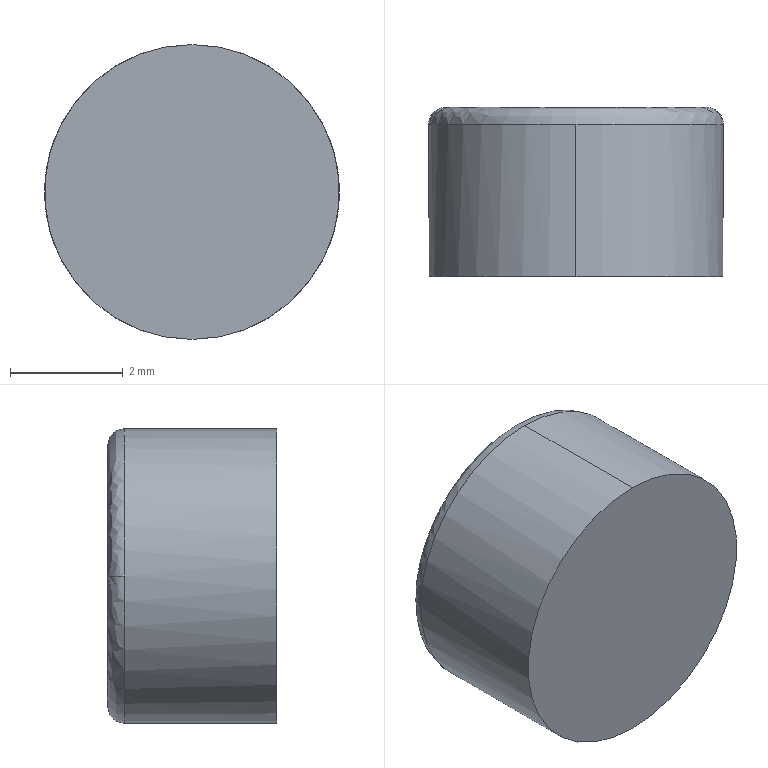Part | SolidWorks | features BaseBody 1 | 1 solid | 19 faces | box 5.232 x 3 x 5.232 mm | volume 54.683 mm3 | plane 15 | spline 2 | cylinder 2 | commonest cylinder face diameters 5.232 x2
STEP:
#1=CARTESIAN_POINT('',(15.184,100.1,10.6));
#2=VERTEX_POINT('',#1);
#3=CARTESIAN_POINT('',(19.816,100.1,10.6));
#4=VERTEX_POINT('',#3);
#5=CARTESIAN_POINT('',(15.184,100.1,10.6));
#6=CARTESIAN_POINT('',(15.184,100.1,5.968));
#7=CARTESIAN_POINT('',(19.816,100.1,5.968));
#8=CARTESIAN_POINT('',(19.816,100.1,10.6));
#9=(BOUNDED_CURVE()B_SPLINE_CURVE(3,(#5,#6,#7,#8),.UNSPECIFIED.,.F.,.T.)B_SPLINE_CURVE_WITH_KNOTS((4,4),(0.,1.),.UNSPECIFIED.)CURVE()GEOMETRIC_REPRESENTATION_ITEM()RATIONAL_B_SPLINE_CURVE((1.,0.3333,0.3333,1.))REPRESENTATION_ITEM(''));
#10=EDGE_CURVE('',#2,#4,#9,.T.);
#11=ORIENTED_EDGE('',*,*,#10,.T.);
#12=CARTESIAN_POINT('',(20.116,99.8,10.6));
#13=VERTEX_POINT('',#12);
#14=CARTESIAN_POINT('',(19.816,99.8,10.6));
#15=DIRECTION('',(0.,0.,-1.));
#16=DIRECTION('',(1.,0.,0.));
#17=AXIS2_PLACEMENT_3D('',#14,#15,#16);
#18=CIRCLE('',#17,0.3);
#19=EDGE_CURVE('',#4,#13,#18,.T.);
#20=ORIENTED_EDGE('',*,*,#19,.T.);
#21=CARTESIAN_POINT('',(17.5,99.8,7.984));
#22=VERTEX_POINT('',#21);
#23=CARTESIAN_POINT('',(17.5,99.8,10.6));
#24=DIRECTION('',(0.,-1.,0.));
#25=DIRECTION('',(0.,0.,1.));
#26=AXIS2_PLACEMENT_3D('',#23,#24,#25);
#27=CIRCLE('',#26,2.616);
#28=EDGE_CURVE('',#22,#13,#27,.T.);
#29=ORIENTED_EDGE('',*,*,#28,.F.);
#30=CARTESIAN_POINT('',(14.884,99.8,10.6));
#31=VERTEX_POINT('',#30);
#32=CARTESIAN_POINT('',(17.5,99.8,10.6));
#33=DIRECTION('',(0.,-1.,0.));
#34=DIRECTION('',(0.,0.,1.));
#35=AXIS2_PLACEMENT_3D('',#32,#33,#34);
#36=CIRCLE('',#35,2.616);
#37=EDGE_CURVE('',#31,#22,#36,.T.);
#38=ORIENTED_EDGE('',*,*,#37,.F.);
#39=CARTESIAN_POINT('',(15.184,99.8,10.6));
#40=DIRECTION('',(0.,0.,1.));
#41=DIRECTION('',(-1.,0.,0.));
#42=AXIS2_PLACEMENT_3D('',#39,#40,#41);
#43=CIRCLE('',#42,0.3);
#44=EDGE_CURVE('',#2,#31,#43,.T.);
#45=ORIENTED_EDGE('',*,*,#44,.F.);
#46=EDGE_LOOP('',(#11,#20,#29,#38,#45));
#47=FACE_OUTER_BOUND('',#46,.T.);
#48=CARTESIAN_POINT('',(19.816,100.1,10.6));
#49=CARTESIAN_POINT('',(19.816,100.1,5.968));
#50=CARTESIAN_POINT('',(15.184,100.1,5.968));
#51=CARTESIAN_POINT('',(15.184,100.1,10.6));
#52=CARTESIAN_POINT('',(19.992,100.1,10.6));
#53=CARTESIAN_POINT('',(19.992,100.1,5.617));
#54=CARTESIAN_POINT('',(15.008,100.1,5.617));
#55=CARTESIAN_POINT('',(15.008,100.1,10.6));
#56=CARTESIAN_POINT('',(20.116,99.976,10.6));
#57=CARTESIAN_POINT('',(20.116,99.976,5.368));
#58=CARTESIAN_POINT('',(14.884,99.976,5.368));
#59=CARTESIAN_POINT('',(14.884,99.976,10.6));
#60=CARTESIAN_POINT('',(20.116,99.8,10.6));
#61=CARTESIAN_POINT('',(20.116,99.8,5.368));
#62=CARTESIAN_POINT('',(14.884,99.8,5.368));
#63=CARTESIAN_POINT('',(14.884,99.8,10.6));
#64=(BOUNDED_SURFACE()B_SPLINE_SURFACE(3,3,((#48,#49,#50,#51),(#52,#53,#54,#55),(#56,#57,#58,#59),(#60,#61,#62,#63)),.UNSPECIFIED.,.F.,.F.,.F.)B_SPLINE_SURFACE_WITH_KNOTS((4,4),(4,4),(0.,1.),(0.,1.),.UNSPECIFIED.)GEOMETRIC_REPRESENTATION_ITEM()RATIONAL_B_SPLINE_SURFACE(((1.,0.3333,0.3333,1.),(0.8047,0.2682,0.2682,0.8047),(0.8047,0.2682,0.2682,0.8047),(1.,0.3333,0.3333,1.)))REPRESENTATION_ITEM('')SURFACE());
#65=ADVANCED_FACE('',(#47),#64,.T.);
#66=CARTESIAN_POINT('',(17.5,97.1,13.216));
#67=VERTEX_POINT('',#66);
#68=CARTESIAN_POINT('',(17.5,97.1,7.984));
#69=VERTEX_POINT('',#68);
#70=CARTESIAN_POINT('',(17.5,97.1,10.6));
#71=DIRECTION('',(0.,1.,0.));
#72=DIRECTION('',(0.,0.,1.));
#73=AXIS2_PLACEMENT_3D('',#70,#71,#72);
#74=CIRCLE('',#73,2.616);
#75=EDGE_CURVE('',#67,#69,#74,.T.);
#76=ORIENTED_EDGE('',*,*,#75,.T.);
#77=CARTESIAN_POINT('',(17.5,98.45,7.984));
#78=DIRECTION('',(0.,1.,0.));
#79=VECTOR('',#78,1000.);
#80=LINE('',#77,#79);
#81=EDGE_CURVE('',#69,#22,#80,.T.);
#82=ORIENTED_EDGE('',*,*,#81,.T.);
#83=ORIENTED_EDGE('',*,*,#28,.T.);
#84=CARTESIAN_POINT('',(17.5,99.8,13.216));
#85=VERTEX_POINT('',#84);
#86=CARTESIAN_POINT('',(17.5,99.8,10.6));
#87=DIRECTION('',(0.,-1.,0.));
#88=DIRECTION('',(0.,0.,1.));
#89=AXIS2_PLACEMENT_3D('',#86,#87,#88);
#90=CIRCLE('',#89,2.616);
#91=EDGE_CURVE('',#13,#85,#90,.T.);
#92=ORIENTED_EDGE('',*,*,#91,.T.);
#93=CARTESIAN_POINT('',(17.5,98.45,13.216));
#94=DIRECTION('',(0.,1.,0.));
#95=VECTOR('',#94,1000.);
#96=LINE('',#93,#95);
#97=EDGE_CURVE('',#67,#85,#96,.T.);
#98=ORIENTED_EDGE('',*,*,#97,.F.);
#99=EDGE_LOOP('',(#76,#82,#83,#92,#98));
#100=FACE_OUTER_BOUND('',#99,.T.);
#101=CARTESIAN_POINT('',(17.5,98.45,10.6));
#102=DIRECTION('',(0.,1.,0.));
#103=DIRECTION('',(0.,0.,1.));
#104=AXIS2_PLACEMENT_3D('',#101,#102,#103);
#105=CYLINDRICAL_SURFACE('',#104,2.616);
#106=ADVANCED_FACE('',(#100),#105,.T.);
#107=ORIENTED_EDGE('',*,*,#81,.F.);
#108=CARTESIAN_POINT('',(17.5,97.1,10.6));
#109=DIRECTION('',(0.,1.,0.));
#110=DIRECTION('',(0.,0.,1.));
#111=AXIS2_PLACEMENT_3D('',#108,#109,#110);
#112=CIRCLE('',#111,2.616);
#113=EDGE_CURVE('',#69,#67,#112,.T.);
#114=ORIENTED_EDGE('',*,*,#113,.T.);
#115=ORIENTED_EDGE('',*,*,#97,.T.);
#116=CARTESIAN_POINT('',(17.5,99.8,10.6));
#117=DIRECTION('',(0.,-1.,0.));
#118=DIRECTION('',(0.,0.,1.));
#119=AXIS2_PLACEMENT_3D('',#116,#117,#118);
#120=CIRCLE('',#119,2.616);
#121=EDGE_CURVE('',#85,#31,#120,.T.);
#122=ORIENTED_EDGE('',*,*,#121,.T.);
#123=ORIENTED_EDGE('',*,*,#37,.T.);
#124=EDGE_LOOP('',(#107,#114,#115,#122,#123));
#125=FACE_OUTER_BOUND('',#124,.T.);
#126=CARTESIAN_POINT('',(17.5,98.45,10.6));
#127=DIRECTION('',(0.,1.,0.));
#128=DIRECTION('',(0.,0.,1.));
#129=AXIS2_PLACEMENT_3D('',#126,#127,#128);
#130=CYLINDRICAL_SURFACE('',#129,2.616);
#131=ADVANCED_FACE('',(#125),#130,.T.);
#132=ORIENTED_EDGE('',*,*,#19,.F.);
#133=CARTESIAN_POINT('',(15.184,100.1,10.6));
#134=CARTESIAN_POINT('',(15.184,100.1,10.747));
#135=CARTESIAN_POINT('',(15.204,100.1,10.964));
#136=CARTESIAN_POINT('',(15.264,100.1,11.211));
#137=CARTESIAN_POINT('',(15.302,100.1,11.332));
#138=CARTESIAN_POINT('',(15.321,100.1,11.384));
#139=CARTESIAN_POINT('',(15.333,100.1,11.418));
#140=CARTESIAN_POINT('',(15.339,100.1,11.434));
#141=CARTESIAN_POINT('',(15.464,100.1,11.75));
#142=CARTESIAN_POINT('',(15.637,100.1,12.012));
#143=CARTESIAN_POINT('',(15.975,100.1,12.351));
#144=CARTESIAN_POINT('',(16.158,100.1,12.5));
#145=CARTESIAN_POINT('',(16.395,100.1,12.638));
#146=CARTESIAN_POINT('',(16.519,100.1,12.699));
#147=CARTESIAN_POINT('',(16.574,100.1,12.723));
#148=CARTESIAN_POINT('',(16.61,100.1,12.738));
#149=CARTESIAN_POINT('',(16.63,100.1,12.747));
#150=CARTESIAN_POINT('',(16.921,100.1,12.862));
#151=CARTESIAN_POINT('',(17.206,100.1,12.916));
#152=CARTESIAN_POINT('',(17.647,100.1,12.916));
#153=CARTESIAN_POINT('',(17.864,100.1,12.896));
#154=CARTESIAN_POINT('',(18.11,100.1,12.836));
#155=CARTESIAN_POINT('',(18.232,100.1,12.798));
#156=CARTESIAN_POINT('',(18.284,100.1,12.779));
#157=CARTESIAN_POINT('',(18.318,100.1,12.767));
#158=CARTESIAN_POINT('',(18.334,100.1,12.761));
#159=CARTESIAN_POINT('',(18.65,100.1,12.636));
#160=CARTESIAN_POINT('',(18.912,100.1,12.463));
#161=CARTESIAN_POINT('',(19.251,100.1,12.125));
#162=CARTESIAN_POINT('',(19.4,100.1,11.942));
#163=CARTESIAN_POINT('',(19.538,100.1,11.705));
#164=CARTESIAN_POINT('',(19.599,100.1,11.581));
#165=CARTESIAN_POINT('',(19.623,100.1,11.526));
#166=CARTESIAN_POINT('',(19.638,100.1,11.49));
#167=CARTESIAN_POINT('',(19.647,100.1,11.47));
#168=CARTESIAN_POINT('',(19.762,100.1,11.179));
#169=CARTESIAN_POINT('',(19.816,100.1,10.895));
#170=CARTESIAN_POINT('',(19.816,100.1,10.6));
#171=B_SPLINE_CURVE_WITH_KNOTS('',3,(#133,#134,#135,#136,#137,#138,#139,#140,#141,#142,#143,#144,#145,#146,#147,#148,#149,#150,#151,#152,#153,#154,#155,#156,#157,#158,#159,#160,#161,#162,#163,#164,#165,#166,#167,#168,#169,#170),.UNSPECIFIED.,.F.,.F.,(4,1,1,1,2,2,2,1,1,1,2,2,2,1,1,1,2,2,2,1,1,1,2,2,4),(0.,0.0625,0.09375,0.1094,0.1172,0.125,0.25,0.3125,0.3438,0.3594,0.3672,0.375,0.5,0.5625,0.5938,0.6094,0.6172,0.625,0.75,0.8125,0.8438,0.8594,0.8672,0.875,1.),.UNSPECIFIED.);
#172=EDGE_CURVE('',#2,#4,#171,.T.);
#173=ORIENTED_EDGE('',*,*,#172,.F.);
#174=ORIENTED_EDGE('',*,*,#44,.T.);
#175=ORIENTED_EDGE('',*,*,#121,.F.);
#176=ORIENTED_EDGE('',*,*,#91,.F.);
#177=EDGE_LOOP('',(#132,#173,#174,#175,#176));
#178=FACE_OUTER_BOUND('',#177,.T.);
#179=CARTESIAN_POINT('',(15.184,100.1,10.6));
#180=CARTESIAN_POINT('',(15.184,100.1,15.232));
#181=CARTESIAN_POINT('',(19.816,100.1,15.232));
#182=CARTESIAN_POINT('',(19.816,100.1,10.6));
#183=CARTESIAN_POINT('',(15.008,100.1,10.6));
#184=CARTESIAN_POINT('',(15.008,100.1,15.583));
#185=CARTESIAN_POINT('',(19.992,100.1,15.583));
#186=CARTESIAN_POINT('',(19.992,100.1,10.6));
#187=CARTESIAN_POINT('',(14.884,99.976,10.6));
#188=CARTESIAN_POINT('',(14.884,99.976,15.832));
#189=CARTESIAN_POINT('',(20.116,99.976,15.832));
#190=CARTESIAN_POINT('',(20.116,99.976,10.6));
#191=CARTESIAN_POINT('',(14.884,99.8,10.6));
#192=CARTESIAN_POINT('',(14.884,99.8,15.832));
#193=CARTESIAN_POINT('',(20.116,99.8,15.832));
#194=CARTESIAN_POINT('',(20.116,99.8,10.6));
#195=(BOUNDED_SURFACE()B_SPLINE_SURFACE(3,3,((#179,#180,#181,#182),(#183,#184,#185,#186),(#187,#188,#189,#190),(#191,#192,#193,#194)),.UNSPECIFIED.,.F.,.F.,.T.)B_SPLINE_SURFACE_WITH_KNOTS((4,4),(4,4),(0.,1.),(0.,1.),.UNSPECIFIED.)GEOMETRIC_REPRESENTATION_ITEM()RATIONAL_B_SPLINE_SURFACE(((1.,0.3333,0.3333,1.),(0.8047,0.2682,0.2682,0.8047),(0.8047,0.2682,0.2682,0.8047),(1.,0.3333,0.3333,1.)))REPRESENTATION_ITEM('')SURFACE());
#196=ADVANCED_FACE('',(#178),#195,.T.);
#197=ORIENTED_EDGE('',*,*,#75,.F.);
#198=ORIENTED_EDGE('',*,*,#113,.F.);
#199=EDGE_LOOP('',(#197,#198));
#200=FACE_OUTER_BOUND('',#199,.T.);
#201=CARTESIAN_POINT('',(18.808,97.1,10.6));
#202=DIRECTION('',(0.,-1.,0.));
#203=DIRECTION('',(0.,0.,-1.));
#204=AXIS2_PLACEMENT_3D('',#201,#202,#203);
#205=PLANE('',#204);
#206=ADVANCED_FACE('',(#200),#205,.T.);
#207=ORIENTED_EDGE('',*,*,#10,.F.);
#208=ORIENTED_EDGE('',*,*,#172,.T.);
#209=EDGE_LOOP('',(#207,#208));
#210=FACE_OUTER_BOUND('',#209,.T.);
#211=CARTESIAN_POINT('',(18.19,100.1,11.8));
#212=VERTEX_POINT('',#211);
#213=CARTESIAN_POINT('',(18.187,100.1,11.795));
#214=VERTEX_POINT('',#213);
#215=CARTESIAN_POINT('',(17.845,100.1,11.2));
#216=DIRECTION('',(-0.4985,0.,-0.8669));
#217=VECTOR('',#216,1000.);
#218=LINE('',#215,#217);
#219=EDGE_CURVE('',#212,#214,#218,.T.);
#220=ORIENTED_EDGE('',*,*,#219,.T.);
#221=CARTESIAN_POINT('',(16.806,100.1,11.798));
#222=VERTEX_POINT('',#221);
#223=CARTESIAN_POINT('',(18.187,100.1,11.795));
#224=DIRECTION('',(-1.,0.,0.001764));
#225=VECTOR('',#224,1000.);
#226=LINE('',#223,#225);
#227=EDGE_CURVE('',#214,#222,#226,.T.);
#228=ORIENTED_EDGE('',*,*,#227,.T.);
#229=CARTESIAN_POINT('',(16.809,100.1,11.793));
#230=VERTEX_POINT('',#229);
#231=CARTESIAN_POINT('',(17.153,100.1,11.199));
#232=DIRECTION('',(0.5015,0.,-0.8651));
#233=VECTOR('',#232,1000.);
#234=LINE('',#231,#233);
#235=EDGE_CURVE('',#222,#230,#234,.T.);
#236=ORIENTED_EDGE('',*,*,#235,.T.);
#237=CARTESIAN_POINT('',(16.116,100.1,10.598));
#238=VERTEX_POINT('',#237);
#239=CARTESIAN_POINT('',(16.463,100.1,11.196));
#240=DIRECTION('',(-0.5015,0.,-0.8651));
#241=VECTOR('',#240,1000.);
#242=LINE('',#239,#241);
#243=EDGE_CURVE('',#230,#238,#242,.T.);
#244=ORIENTED_EDGE('',*,*,#243,.T.);
#245=CARTESIAN_POINT('',(16.121,100.1,10.598));
#246=VERTEX_POINT('',#245);
#247=CARTESIAN_POINT('',(16.808,100.1,10.599));
#248=DIRECTION('',(1.,0.,0.001764));
#249=VECTOR('',#248,1000.);
#250=LINE('',#247,#249);
#251=EDGE_CURVE('',#238,#246,#250,.T.);
#252=ORIENTED_EDGE('',*,*,#251,.T.);
#253=CARTESIAN_POINT('',(16.81,100.1,9.4));
#254=VERTEX_POINT('',#253);
#255=CARTESIAN_POINT('',(16.121,100.1,10.598));
#256=DIRECTION('',(0.4985,0.,-0.8669));
#257=VECTOR('',#256,1000.);
#258=LINE('',#255,#257);
#259=EDGE_CURVE('',#246,#254,#258,.T.);
#260=ORIENTED_EDGE('',*,*,#259,.T.);
#261=CARTESIAN_POINT('',(16.813,100.1,9.405));
#262=VERTEX_POINT('',#261);
#263=CARTESIAN_POINT('',(17.155,100.1,10.));
#264=DIRECTION('',(0.4985,0.,0.8669));
#265=VECTOR('',#264,1000.);
#266=LINE('',#263,#265);
#267=EDGE_CURVE('',#254,#262,#266,.T.);
#268=ORIENTED_EDGE('',*,*,#267,.T.);
#269=CARTESIAN_POINT('',(18.194,100.1,9.402));
#270=VERTEX_POINT('',#269);
#271=CARTESIAN_POINT('',(17.502,100.1,9.404));
#272=DIRECTION('',(1.,0.,-0.001764));
#273=VECTOR('',#272,1000.);
#274=LINE('',#271,#273);
#275=EDGE_CURVE('',#262,#270,#274,.T.);
#276=ORIENTED_EDGE('',*,*,#275,.T.);
#277=CARTESIAN_POINT('',(18.191,100.1,9.407));
#278=VERTEX_POINT('',#277);
#279=CARTESIAN_POINT('',(17.847,100.1,10.001));
#280=DIRECTION('',(-0.5015,0.,0.8651));
#281=VECTOR('',#280,1000.);
#282=LINE('',#279,#281);
#283=EDGE_CURVE('',#270,#278,#282,.T.);
#284=ORIENTED_EDGE('',*,*,#283,.T.);
#285=CARTESIAN_POINT('',(18.884,100.1,10.602));
#286=VERTEX_POINT('',#285);
#287=CARTESIAN_POINT('',(18.537,100.1,10.004));
#288=DIRECTION('',(0.5015,0.,0.8651));
#289=VECTOR('',#288,1000.);
#290=LINE('',#287,#289);
#291=EDGE_CURVE('',#278,#286,#290,.T.);
#292=ORIENTED_EDGE('',*,*,#291,.T.);
#293=CARTESIAN_POINT('',(18.879,100.1,10.602));
#294=VERTEX_POINT('',#293);
#295=CARTESIAN_POINT('',(18.192,100.1,10.601));
#296=DIRECTION('',(-1.,0.,-0.001764));
#297=VECTOR('',#296,1000.);
#298=LINE('',#295,#297);
#299=EDGE_CURVE('',#286,#294,#298,.T.);
#300=ORIENTED_EDGE('',*,*,#299,.T.);
#301=CARTESIAN_POINT('',(18.879,100.1,10.602));
#302=DIRECTION('',(-0.4985,0.,0.8669));
#303=VECTOR('',#302,1000.);
#304=LINE('',#301,#303);
#305=EDGE_CURVE('',#294,#212,#304,.T.);
#306=ORIENTED_EDGE('',*,*,#305,.T.);
#307=EDGE_LOOP('',(#220,#228,#236,#244,#252,#260,#268,#276,#284,#292,#300,#306));
#308=FACE_BOUND('',#307,.T.);
#309=CARTESIAN_POINT('',(18.658,100.1,10.6));
#310=DIRECTION('',(0.,1.,0.));
#311=DIRECTION('',(0.,0.,1.));
#312=AXIS2_PLACEMENT_3D('',#309,#310,#311);
#313=PLANE('',#312);
#314=ADVANCED_FACE('',(#210,#308),#313,.T.);
#315=CARTESIAN_POINT('',(16.806,98.18,11.798));
#316=VERTEX_POINT('',#315);
#317=CARTESIAN_POINT('',(18.187,98.18,11.795));
#318=VERTEX_POINT('',#317);
#319=CARTESIAN_POINT('',(17.498,98.18,11.796));
#320=DIRECTION('',(1.,0.,-0.001764));
#321=VECTOR('',#320,1000.);
#322=LINE('',#319,#321);
#323=EDGE_CURVE('',#316,#318,#322,.T.);
#324=ORIENTED_EDGE('',*,*,#323,.F.);
#325=CARTESIAN_POINT('',(16.806,98.18,11.798));
#326=DIRECTION('',(0.,-1.,0.));
#327=VECTOR('',#326,1000.);
#328=LINE('',#325,#327);
#329=EDGE_CURVE('',#222,#316,#328,.T.);
#330=ORIENTED_EDGE('',*,*,#329,.F.);
#331=ORIENTED_EDGE('',*,*,#227,.F.);
#332=CARTESIAN_POINT('',(18.187,98.18,11.795));
#333=DIRECTION('',(0.,1.,0.));
#334=VECTOR('',#333,1000.);
#335=LINE('',#332,#334);
#336=EDGE_CURVE('',#318,#214,#335,.T.);
#337=ORIENTED_EDGE('',*,*,#336,.F.);
#338=EDGE_LOOP('',(#324,#330,#331,#337));
#339=FACE_OUTER_BOUND('',#338,.T.);
#340=CARTESIAN_POINT('',(17.498,98.18,11.796));
#341=DIRECTION('',(0.001764,0.,1.));
#342=DIRECTION('',(1.,0.,-0.001764));
#343=AXIS2_PLACEMENT_3D('',#340,#341,#342);
#344=PLANE('',#343);
#345=ADVANCED_FACE('',(#339),#344,.F.);
#346=ORIENTED_EDGE('',*,*,#219,.F.);
#347=CARTESIAN_POINT('',(18.19,98.18,11.8));
#348=VERTEX_POINT('',#347);
#349=CARTESIAN_POINT('',(18.19,98.18,11.8));
#350=DIRECTION('',(0.,1.,0.));
#351=VECTOR('',#350,1000.);
#352=LINE('',#349,#351);
#353=EDGE_CURVE('',#348,#212,#352,.T.);
#354=ORIENTED_EDGE('',*,*,#353,.F.);
#355=CARTESIAN_POINT('',(17.845,98.18,11.2));
#356=DIRECTION('',(0.4985,0.,0.8669));
#357=VECTOR('',#356,1000.);
#358=LINE('',#355,#357);
#359=EDGE_CURVE('',#318,#348,#358,.T.);
#360=ORIENTED_EDGE('',*,*,#359,.F.);
#361=ORIENTED_EDGE('',*,*,#336,.T.);
#362=EDGE_LOOP('',(#346,#354,#360,#361));
#363=FACE_OUTER_BOUND('',#362,.T.);
#364=CARTESIAN_POINT('',(17.845,98.18,11.2));
#365=DIRECTION('',(-0.8669,0.,0.4985));
#366=DIRECTION('',(0.4985,0.,0.8669));
#367=AXIS2_PLACEMENT_3D('',#364,#365,#366);
#368=PLANE('',#367);
#369=ADVANCED_FACE('',(#363),#368,.F.);
#370=CARTESIAN_POINT('',(16.81,98.18,9.4));
#371=VERTEX_POINT('',#370);
#372=CARTESIAN_POINT('',(16.121,98.18,10.598));
#373=VERTEX_POINT('',#372);
#374=CARTESIAN_POINT('',(16.465,98.18,10.));
#375=DIRECTION('',(-0.4985,0.,0.8669));
#376=VECTOR('',#375,1000.);
#377=LINE('',#374,#376);
#378=EDGE_CURVE('',#371,#373,#377,.T.);
#379=ORIENTED_EDGE('',*,*,#378,.T.);
#380=CARTESIAN_POINT('',(16.116,98.18,10.598));
#381=VERTEX_POINT('',#380);
#382=CARTESIAN_POINT('',(18.191,98.18,10.601));
#383=DIRECTION('',(-1.,0.,-0.001764));
#384=VECTOR('',#383,1000.);
#385=LINE('',#382,#384);
#386=EDGE_CURVE('',#373,#381,#385,.T.);
#387=ORIENTED_EDGE('',*,*,#386,.T.);
#388=CARTESIAN_POINT('',(16.809,98.18,11.793));
#389=VERTEX_POINT('',#388);
#390=CARTESIAN_POINT('',(16.463,98.18,11.196));
#391=DIRECTION('',(0.5015,0.,0.8651));
#392=VECTOR('',#391,1000.);
#393=LINE('',#390,#392);
#394=EDGE_CURVE('',#381,#389,#393,.T.);
#395=ORIENTED_EDGE('',*,*,#394,.T.);
#396=CARTESIAN_POINT('',(16.809,98.18,11.793));
#397=DIRECTION('',(-0.5015,0.,0.8651));
#398=VECTOR('',#397,1000.);
#399=LINE('',#396,#398);
#400=EDGE_CURVE('',#389,#316,#399,.T.);
#401=ORIENTED_EDGE('',*,*,#400,.T.);
#402=ORIENTED_EDGE('',*,*,#323,.T.);
#403=ORIENTED_EDGE('',*,*,#359,.T.);
#404=CARTESIAN_POINT('',(18.879,98.18,10.602));
#405=VERTEX_POINT('',#404);
#406=CARTESIAN_POINT('',(18.19,98.18,11.8));
#407=DIRECTION('',(0.4985,0.,-0.8669));
#408=VECTOR('',#407,1000.);
#409=LINE('',#406,#408);
#410=EDGE_CURVE('',#348,#405,#409,.T.);
#411=ORIENTED_EDGE('',*,*,#410,.T.);
#412=CARTESIAN_POINT('',(18.884,98.18,10.602));
#413=VERTEX_POINT('',#412);
#414=CARTESIAN_POINT('',(18.191,98.18,10.601));
#415=DIRECTION('',(1.,0.,0.001764));
#416=VECTOR('',#415,1000.);
#417=LINE('',#414,#416);
#418=EDGE_CURVE('',#405,#413,#417,.T.);
#419=ORIENTED_EDGE('',*,*,#418,.T.);
#420=CARTESIAN_POINT('',(18.191,98.18,9.407));
#421=VERTEX_POINT('',#420);
#422=CARTESIAN_POINT('',(18.537,98.18,10.004));
#423=DIRECTION('',(-0.5015,0.,-0.8651));
#424=VECTOR('',#423,1000.);
#425=LINE('',#422,#424);
#426=EDGE_CURVE('',#413,#421,#425,.T.);
#427=ORIENTED_EDGE('',*,*,#426,.T.);
#428=CARTESIAN_POINT('',(18.194,98.18,9.402));
#429=VERTEX_POINT('',#428);
#430=CARTESIAN_POINT('',(17.847,98.18,10.001));
#431=DIRECTION('',(0.5015,0.,-0.8651));
#432=VECTOR('',#431,1000.);
#433=LINE('',#430,#432);
#434=EDGE_CURVE('',#421,#429,#433,.T.);
#435=ORIENTED_EDGE('',*,*,#434,.T.);
#436=CARTESIAN_POINT('',(16.813,98.18,9.405));
#437=VERTEX_POINT('',#436);
#438=CARTESIAN_POINT('',(17.502,98.18,9.404));
#439=DIRECTION('',(-1.,0.,0.001764));
#440=VECTOR('',#439,1000.);
#441=LINE('',#438,#440);
#442=EDGE_CURVE('',#429,#437,#441,.T.);
#443=ORIENTED_EDGE('',*,*,#442,.T.);
#444=CARTESIAN_POINT('',(17.155,98.18,10.));
#445=DIRECTION('',(-0.4985,0.,-0.8669));
#446=VECTOR('',#445,1000.);
#447=LINE('',#444,#446);
#448=EDGE_CURVE('',#437,#371,#447,.T.);
#449=ORIENTED_EDGE('',*,*,#448,.T.);
#450=EDGE_LOOP('',(#379,#387,#395,#401,#402,#403,#411,#419,#427,#435,#443,#449));
#451=FACE_OUTER_BOUND('',#450,.T.);
#452=CARTESIAN_POINT('',(18.19,98.18,11.));
#453=DIRECTION('',(0.,1.,0.));
#454=DIRECTION('',(0.,0.,1.));
#455=AXIS2_PLACEMENT_3D('',#452,#453,#454);
#456=PLANE('',#455);
#457=ADVANCED_FACE('',(#451),#456,.T.);
#458=ORIENTED_EDGE('',*,*,#235,.F.);
#459=ORIENTED_EDGE('',*,*,#329,.T.);
#460=ORIENTED_EDGE('',*,*,#400,.F.);
#461=CARTESIAN_POINT('',(16.809,98.18,11.793));
#462=DIRECTION('',(0.,-1.,0.));
#463=VECTOR('',#462,1000.);
#464=LINE('',#461,#463);
#465=EDGE_CURVE('',#230,#389,#464,.T.);
#466=ORIENTED_EDGE('',*,*,#465,.F.);
#467=EDGE_LOOP('',(#458,#459,#460,#466));
#468=FACE_OUTER_BOUND('',#467,.T.);
#469=CARTESIAN_POINT('',(17.153,98.18,11.199));
#470=DIRECTION('',(-0.8651,0.,-0.5015));
#471=DIRECTION('',(-0.5015,0.,0.8651));
#472=AXIS2_PLACEMENT_3D('',#469,#470,#471);
#473=PLANE('',#472);
#474=ADVANCED_FACE('',(#468),#473,.F.);
#475=ORIENTED_EDGE('',*,*,#410,.F.);
#476=ORIENTED_EDGE('',*,*,#353,.T.);
#477=ORIENTED_EDGE('',*,*,#305,.F.);
#478=CARTESIAN_POINT('',(18.879,98.18,10.602));
#479=DIRECTION('',(0.,1.,0.));
#480=VECTOR('',#479,1000.);
#481=LINE('',#478,#480);
#482=EDGE_CURVE('',#405,#294,#481,.T.);
#483=ORIENTED_EDGE('',*,*,#482,.F.);
#484=EDGE_LOOP('',(#475,#476,#477,#483));
#485=FACE_OUTER_BOUND('',#484,.T.);
#486=CARTESIAN_POINT('',(18.535,98.18,11.2));
#487=DIRECTION('',(0.8669,0.,0.4985));
#488=DIRECTION('',(0.4985,0.,-0.8669));
#489=AXIS2_PLACEMENT_3D('',#486,#487,#488);
#490=PLANE('',#489);
#491=ADVANCED_FACE('',(#485),#490,.F.);
#492=ORIENTED_EDGE('',*,*,#394,.F.);
#493=CARTESIAN_POINT('',(16.116,98.18,10.598));
#494=DIRECTION('',(0.,-1.,0.));
#495=VECTOR('',#494,1000.);
#496=LINE('',#493,#495);
#497=EDGE_CURVE('',#238,#381,#496,.T.);
#498=ORIENTED_EDGE('',*,*,#497,.F.);
#499=ORIENTED_EDGE('',*,*,#243,.F.);
#500=ORIENTED_EDGE('',*,*,#465,.T.);
#501=EDGE_LOOP('',(#492,#498,#499,#500));
#502=FACE_OUTER_BOUND('',#501,.T.);
#503=CARTESIAN_POINT('',(16.463,98.18,11.196));
#504=DIRECTION('',(-0.8651,0.,0.5015));
#505=DIRECTION('',(0.5015,0.,0.8651));
#506=AXIS2_PLACEMENT_3D('',#503,#504,#505);
#507=PLANE('',#506);
#508=ADVANCED_FACE('',(#502),#507,.F.);
#509=ORIENTED_EDGE('',*,*,#299,.F.);
#510=CARTESIAN_POINT('',(18.884,98.18,10.602));
#511=DIRECTION('',(0.,1.,0.));
#512=VECTOR('',#511,1000.);
#513=LINE('',#510,#512);
#514=EDGE_CURVE('',#413,#286,#513,.T.);
#515=ORIENTED_EDGE('',*,*,#514,.F.);
#516=ORIENTED_EDGE('',*,*,#418,.F.);
#517=ORIENTED_EDGE('',*,*,#482,.T.);
#518=EDGE_LOOP('',(#509,#515,#516,#517));
#519=FACE_OUTER_BOUND('',#518,.T.);
#520=CARTESIAN_POINT('',(18.192,98.18,10.601));
#521=DIRECTION('',(-0.001764,0.,1.));
#522=DIRECTION('',(1.,0.,0.001764));
#523=AXIS2_PLACEMENT_3D('',#520,#521,#522);
#524=PLANE('',#523);
#525=ADVANCED_FACE('',(#519),#524,.F.);
#526=ORIENTED_EDGE('',*,*,#251,.F.);
#527=ORIENTED_EDGE('',*,*,#497,.T.);
#528=ORIENTED_EDGE('',*,*,#386,.F.);
#529=CARTESIAN_POINT('',(16.121,98.18,10.598));
#530=DIRECTION('',(0.,-1.,0.));
#531=VECTOR('',#530,1000.);
#532=LINE('',#529,#531);
#533=EDGE_CURVE('',#246,#373,#532,.T.);
#534=ORIENTED_EDGE('',*,*,#533,.F.);
#535=EDGE_LOOP('',(#526,#527,#528,#534));
#536=FACE_OUTER_BOUND('',#535,.T.);
#537=CARTESIAN_POINT('',(16.808,98.18,10.599));
#538=DIRECTION('',(0.001764,0.,-1.));
#539=DIRECTION('',(-1.,0.,-0.001764));
#540=AXIS2_PLACEMENT_3D('',#537,#538,#539);
#541=PLANE('',#540);
#542=ADVANCED_FACE('',(#536),#541,.F.);
#543=ORIENTED_EDGE('',*,*,#426,.F.);
#544=ORIENTED_EDGE('',*,*,#514,.T.);
#545=ORIENTED_EDGE('',*,*,#291,.F.);
#546=CARTESIAN_POINT('',(18.191,98.18,9.407));
#547=DIRECTION('',(0.,1.,0.));
#548=VECTOR('',#547,1000.);
#549=LINE('',#546,#548);
#550=EDGE_CURVE('',#421,#278,#549,.T.);
#551=ORIENTED_EDGE('',*,*,#550,.F.);
#552=EDGE_LOOP('',(#543,#544,#545,#551));
#553=FACE_OUTER_BOUND('',#552,.T.);
#554=CARTESIAN_POINT('',(18.537,98.18,10.004));
#555=DIRECTION('',(0.8651,0.,-0.5015));
#556=DIRECTION('',(-0.5015,0.,-0.8651));
#557=AXIS2_PLACEMENT_3D('',#554,#555,#556);
#558=PLANE('',#557);
#559=ADVANCED_FACE('',(#553),#558,.F.);
#560=ORIENTED_EDGE('',*,*,#378,.F.);
#561=CARTESIAN_POINT('',(16.81,98.18,9.4));
#562=DIRECTION('',(0.,-1.,0.));
#563=VECTOR('',#562,1000.);
#564=LINE('',#561,#563);
#565=EDGE_CURVE('',#254,#371,#564,.T.);
#566=ORIENTED_EDGE('',*,*,#565,.F.);
#567=ORIENTED_EDGE('',*,*,#259,.F.);
#568=ORIENTED_EDGE('',*,*,#533,.T.);
#569=EDGE_LOOP('',(#560,#566,#567,#568));
#570=FACE_OUTER_BOUND('',#569,.T.);
#571=CARTESIAN_POINT('',(16.465,98.18,10.));
#572=DIRECTION('',(-0.8669,0.,-0.4985));
#573=DIRECTION('',(-0.4985,0.,0.8669));
#574=AXIS2_PLACEMENT_3D('',#571,#572,#573);
#575=PLANE('',#574);
#576=ADVANCED_FACE('',(#570),#575,.F.);
#577=ORIENTED_EDGE('',*,*,#283,.F.);
#578=CARTESIAN_POINT('',(18.194,98.18,9.402));
#579=DIRECTION('',(0.,1.,0.));
#580=VECTOR('',#579,1000.);
#581=LINE('',#578,#580);
#582=EDGE_CURVE('',#429,#270,#581,.T.);
#583=ORIENTED_EDGE('',*,*,#582,.F.);
#584=ORIENTED_EDGE('',*,*,#434,.F.);
#585=ORIENTED_EDGE('',*,*,#550,.T.);
#586=EDGE_LOOP('',(#577,#583,#584,#585));
#587=FACE_OUTER_BOUND('',#586,.T.);
#588=CARTESIAN_POINT('',(17.847,98.18,10.001));
#589=DIRECTION('',(0.8651,0.,0.5015));
#590=DIRECTION('',(0.5015,0.,-0.8651));
#591=AXIS2_PLACEMENT_3D('',#588,#589,#590);
#592=PLANE('',#591);
#593=ADVANCED_FACE('',(#587),#592,.F.);
#594=ORIENTED_EDGE('',*,*,#267,.F.);
#595=ORIENTED_EDGE('',*,*,#565,.T.);
#596=ORIENTED_EDGE('',*,*,#448,.F.);
#597=CARTESIAN_POINT('',(16.813,98.18,9.405));
#598=DIRECTION('',(0.,-1.,0.));
#599=VECTOR('',#598,1000.);
#600=LINE('',#597,#599);
#601=EDGE_CURVE('',#262,#437,#600,.T.);
#602=ORIENTED_EDGE('',*,*,#601,.F.);
#603=EDGE_LOOP('',(#594,#595,#596,#602));
#604=FACE_OUTER_BOUND('',#603,.T.);
#605=CARTESIAN_POINT('',(17.155,98.18,10.));
#606=DIRECTION('',(0.8669,0.,-0.4985));
#607=DIRECTION('',(-0.4985,0.,-0.8669));
#608=AXIS2_PLACEMENT_3D('',#605,#606,#607);
#609=PLANE('',#608);
#610=ADVANCED_FACE('',(#604),#609,.F.);
#611=ORIENTED_EDGE('',*,*,#442,.F.);
#612=ORIENTED_EDGE('',*,*,#582,.T.);
#613=ORIENTED_EDGE('',*,*,#275,.F.);
#614=ORIENTED_EDGE('',*,*,#601,.T.);
#615=EDGE_LOOP('',(#611,#612,#613,#614));
#616=FACE_OUTER_BOUND('',#615,.T.);
#617=CARTESIAN_POINT('',(17.502,98.18,9.404));
#618=DIRECTION('',(-0.001764,0.,-1.));
#619=DIRECTION('',(-1.,0.,0.001764));
#620=AXIS2_PLACEMENT_3D('',#617,#618,#619);
#621=PLANE('',#620);
#622=ADVANCED_FACE('',(#616),#621,.F.);
#623=CLOSED_SHELL('',(#65,#106,#131,#196,#206,#314,#345,#369,#457,#474,#491,#508,#525,#542,#559,#576,#593,#610,#622));
#624=MANIFOLD_SOLID_BREP('',#623);
#625=CARTESIAN_POINT('',(0.,0.,0.));
#626=DIRECTION('',(0.,0.,1.));
#627=DIRECTION('',(1.,0.,0.));
#628=AXIS2_PLACEMENT_3D('',#625,#626,#627);
#629=(LENGTH_UNIT()NAMED_UNIT(*)SI_UNIT(.MILLI.,.METRE.));
#630=UNCERTAINTY_MEASURE_WITH_UNIT(LENGTH_MEASURE(0.00001),#629,'','');
#631=(NAMED_UNIT(*)PLANE_ANGLE_UNIT()SI_UNIT($,.RADIAN.));
#632=(NAMED_UNIT(*)SI_UNIT($,.STERADIAN.)SOLID_ANGLE_UNIT());
#633=(GEOMETRIC_REPRESENTATION_CONTEXT(3)GLOBAL_UNCERTAINTY_ASSIGNED_CONTEXT((#630))GLOBAL_UNIT_ASSIGNED_CONTEXT((#629,#631,#632))REPRESENTATION_CONTEXT('',''));
#634=ADVANCED_BREP_SHAPE_REPRESENTATION('',(#624,#628),#633);